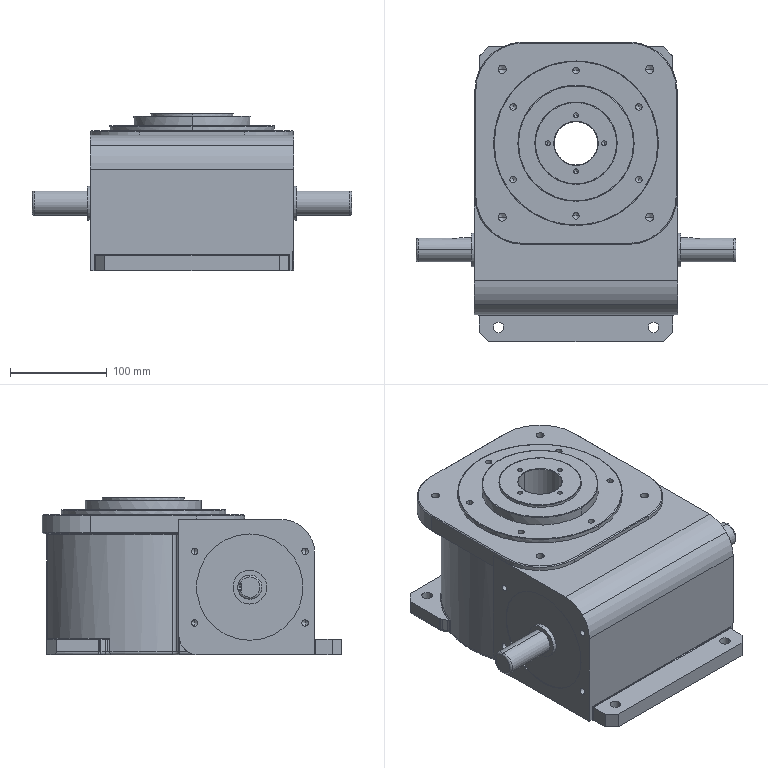Part | SolidWorks | features BaseBody 1 | 1 solid | 376 faces | box 330 x 309.5 x 163 mm | volume 7808751 mm3 | cylinder 136 | plane 115 | cone 54 | torus 39 | spline 32 | commonest cylinder face diameters 6.647 x28 6 x20 2 x16 10 x12 4.917 x8 8.376 x8